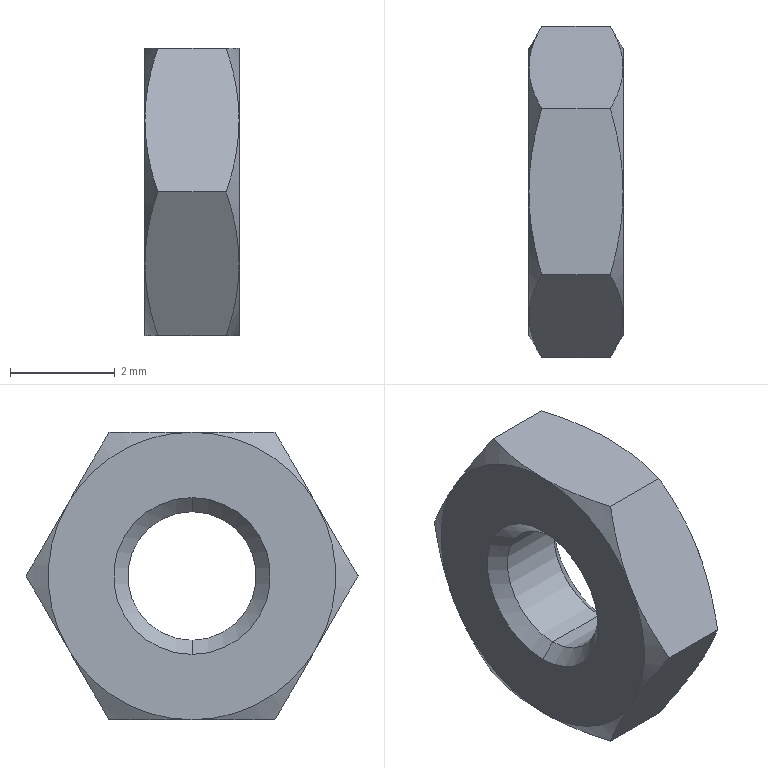Part | STEP file | 0246_Z_009_SAIPOZ3-20_2 | 1 solid | 26 faces | box 1.8 x 6.351 x 5.5 mm | volume 37.634 mm3 | cone 16 | plane 8 | cylinder 2 | commonest cylinder face diameters 2.459 x2